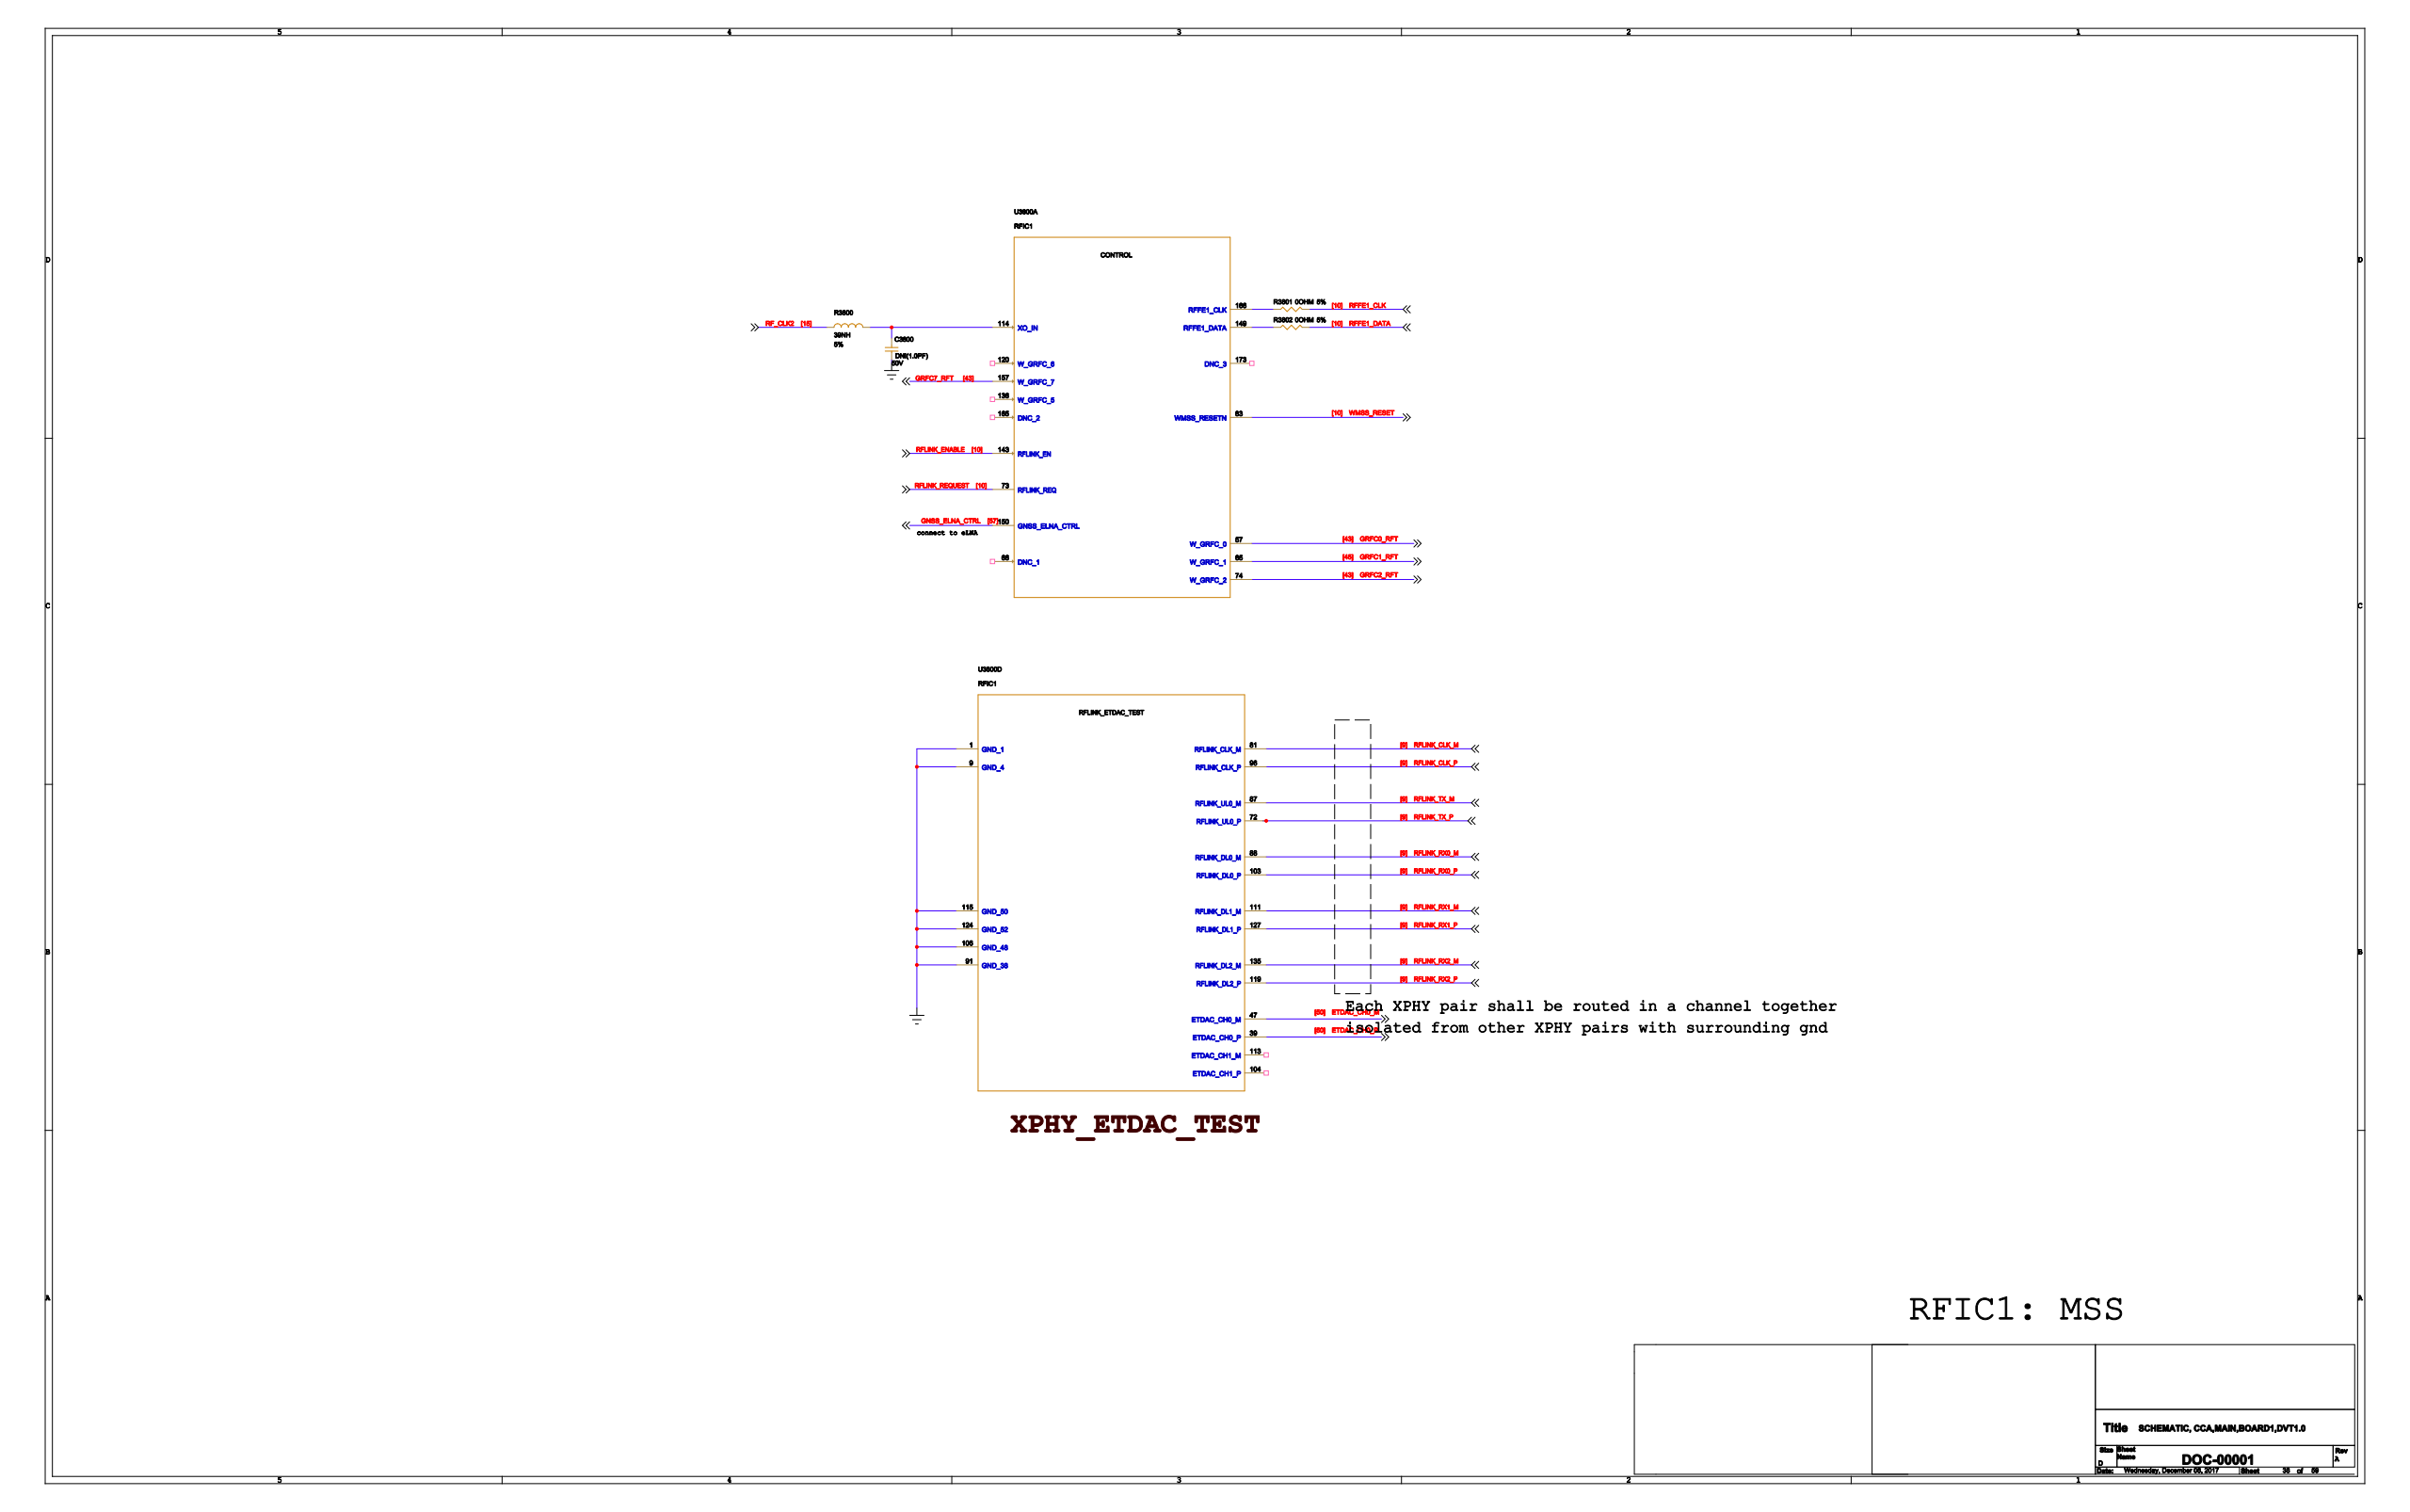Circuit board | KiCad | 1657 parts | 1365 nets | one sheet of the schematic
Parts on this sheet (reference | value | footprint):
C3800
R3800
R3801
R3802
U3800
Nets of these parts (net: part-pin ...):
GND: C3800-1 U3800-1 U3800-4 U3800-9 U3800-91 U3800-106 U3800-115 U3800-124
GNSS_ELNA_CTRL: U3800-150
RFLINK_REQUEST: U3800-73
RFLINK_ENABLE: U3800-143
RFLINK_RX0_P: U3800-103
WMSS_RESET: U3800-83
RFFE1_DATA: R3802-1
RFLINK_RX1_P: U3800-127
RFLINK_RX0_M: U3800-88
RFLINK_TX_M: U3800-87
RFFE1_CLK: R3801-1
RFLINK_RX2_M: U3800-135
RFLINK_RX1_M: U3800-111
RFLINK_CLK_P: U3800-96
RFLINK_TX_P: U3800-72
RFLINK_RX2_P: U3800-119
RFLINK_CLK_M: U3800-81
ETDAC_CH0_M: U3800-47
ETDAC_CH0_P: U3800-39
GRFC2_RFT: U3800-74
GRFC0_RFT: U3800-57
GRFC7_RFT: U3800-157
GRFC1_RFT: U3800-65
N23245910: C3800-2 R3800-2 U3800-114
N42332185: R3802-2 U3800-149
N42332179: R3801-2 U3800-166
RF_CLK2: R3800-1